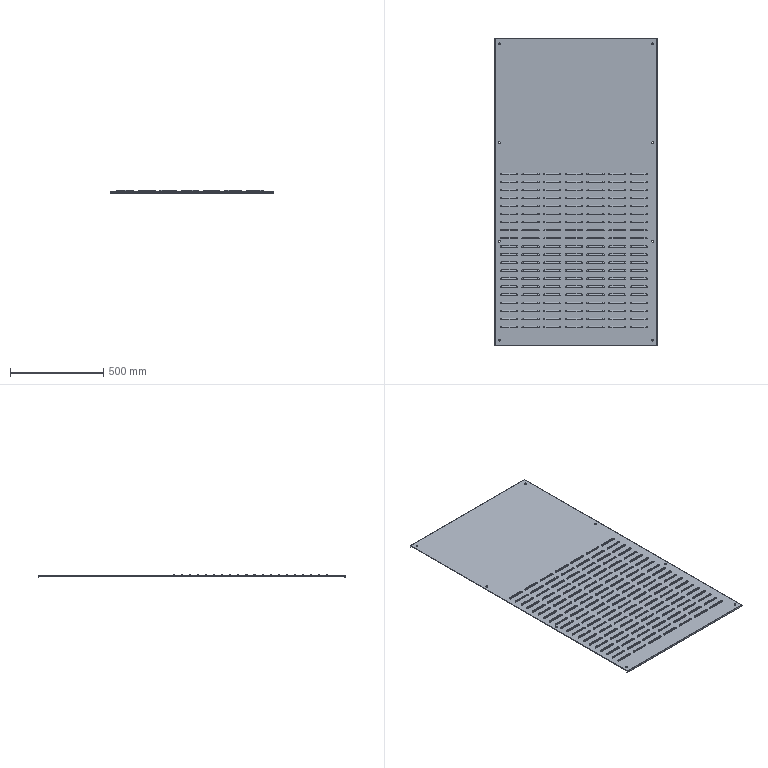Part | SolidWorks | features ICE 5, Fillet 3, LPattern 2, Shell 2, CombineBodies 1, Extrusion 1 | 1 solid | 1574 faces | box 870 x 1650 x 17.75 mm | volume 2197633 mm3 | cylinder 580 | sphere 560 | plane 434 | commonest cylinder face diameters 13.351 x280 13.5 x140 15.5 x140 10 x16 2 x4